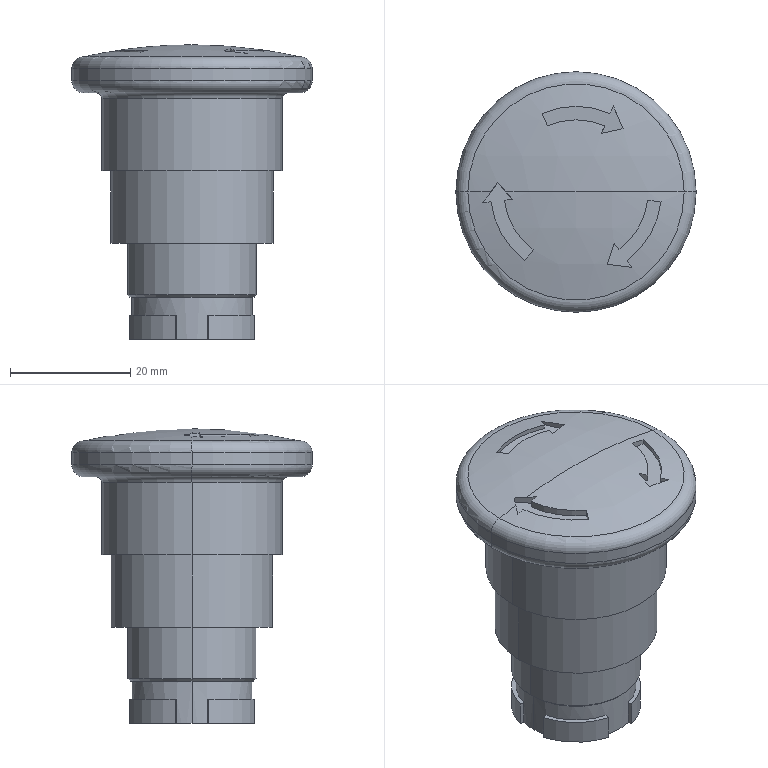Part | STEP file | 001. Schneider red emergency stop switch XB2-BS542C | 1 solid | 68 faces | box 40 x 40 x 49 mm | volume 26880 mm3 | plane 36 | cylinder 22 | torus 6 | sphere 2 | cone 2 | commonest cylinder face diameters 21.5 x6 24 x3 28.5 x3 18 x2 20 x2 27 x2